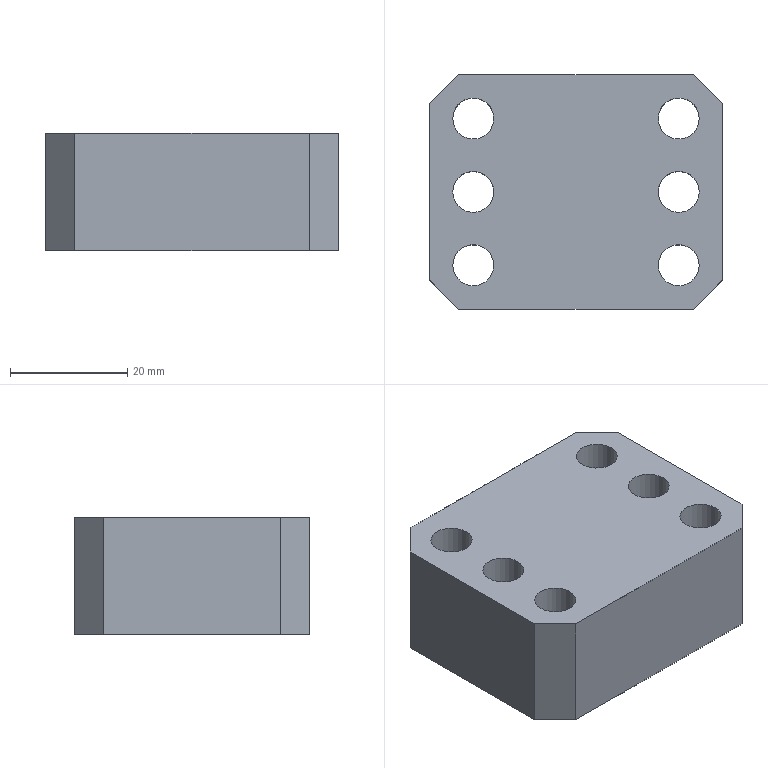Part | NX | features BREP 1 | 1 solid | 16 faces | box 50 x 40 x 20 mm | volume 34382 mm3 | plane 10 | cylinder 6 | commonest cylinder face diameters 7 x6
STEP:
#1=CARTESIAN_POINT('',(25.,-15.,0.));
#2=VERTEX_POINT('',#1);
#3=CARTESIAN_POINT('',(25.,15.,0.));
#4=VERTEX_POINT('',#3);
#5=CARTESIAN_POINT('',(25.,20.,0.));
#6=DIRECTION('',(0.,1.,0.));
#7=VECTOR('',#6,1000.);
#8=LINE('',#5,#7);
#9=EDGE_CURVE('',#2,#4,#8,.T.);
#10=ORIENTED_EDGE('',*,*,#9,.T.);
#11=CARTESIAN_POINT('',(25.,15.,20.));
#12=VERTEX_POINT('',#11);
#13=CARTESIAN_POINT('',(25.,15.,20.));
#14=DIRECTION('',(0.,0.,1.));
#15=VECTOR('',#14,1000.);
#16=LINE('',#13,#15);
#17=EDGE_CURVE('',#4,#12,#16,.T.);
#18=ORIENTED_EDGE('',*,*,#17,.T.);
#19=CARTESIAN_POINT('',(25.,-15.,20.));
#20=VERTEX_POINT('',#19);
#21=CARTESIAN_POINT('',(25.,20.,20.));
#22=DIRECTION('',(0.,1.,0.));
#23=VECTOR('',#22,1000.);
#24=LINE('',#21,#23);
#25=EDGE_CURVE('',#20,#12,#24,.T.);
#26=ORIENTED_EDGE('',*,*,#25,.F.);
#27=CARTESIAN_POINT('',(25.,-15.,20.));
#28=DIRECTION('',(0.,0.,-1.));
#29=VECTOR('',#28,1000.);
#30=LINE('',#27,#29);
#31=EDGE_CURVE('',#20,#2,#30,.T.);
#32=ORIENTED_EDGE('',*,*,#31,.T.);
#33=EDGE_LOOP('',(#10,#18,#26,#32));
#34=FACE_BOUND('',#33,.T.);
#35=CARTESIAN_POINT('',(25.,20.,20.));
#36=DIRECTION('',(-1.,0.,0.));
#37=DIRECTION('',(0.,1.,0.));
#38=AXIS2_PLACEMENT_3D('',#35,#36,#37);
#39=PLANE('',#38);
#40=ADVANCED_FACE('',(#34),#39,.F.);
#41=CARTESIAN_POINT('',(20.,20.,0.));
#42=VERTEX_POINT('',#41);
#43=CARTESIAN_POINT('',(-20.,20.,0.));
#44=VERTEX_POINT('',#43);
#45=CARTESIAN_POINT('',(-25.,20.,0.));
#46=DIRECTION('',(-1.,0.,0.));
#47=VECTOR('',#46,1000.);
#48=LINE('',#45,#47);
#49=EDGE_CURVE('',#42,#44,#48,.T.);
#50=ORIENTED_EDGE('',*,*,#49,.T.);
#51=CARTESIAN_POINT('',(-20.,20.,20.));
#52=VERTEX_POINT('',#51);
#53=CARTESIAN_POINT('',(-20.,20.,20.));
#54=DIRECTION('',(0.,0.,1.));
#55=VECTOR('',#54,1000.);
#56=LINE('',#53,#55);
#57=EDGE_CURVE('',#44,#52,#56,.T.);
#58=ORIENTED_EDGE('',*,*,#57,.T.);
#59=CARTESIAN_POINT('',(20.,20.,20.));
#60=VERTEX_POINT('',#59);
#61=CARTESIAN_POINT('',(-25.,20.,20.));
#62=DIRECTION('',(-1.,0.,0.));
#63=VECTOR('',#62,1000.);
#64=LINE('',#61,#63);
#65=EDGE_CURVE('',#60,#52,#64,.T.);
#66=ORIENTED_EDGE('',*,*,#65,.F.);
#67=CARTESIAN_POINT('',(20.,20.,20.));
#68=DIRECTION('',(0.,0.,-1.));
#69=VECTOR('',#68,1000.);
#70=LINE('',#67,#69);
#71=EDGE_CURVE('',#60,#42,#70,.T.);
#72=ORIENTED_EDGE('',*,*,#71,.T.);
#73=EDGE_LOOP('',(#50,#58,#66,#72));
#74=FACE_BOUND('',#73,.T.);
#75=CARTESIAN_POINT('',(-25.,20.,20.));
#76=DIRECTION('',(0.,-1.,0.));
#77=DIRECTION('',(0.,0.,1.));
#78=AXIS2_PLACEMENT_3D('',#75,#76,#77);
#79=PLANE('',#78);
#80=ADVANCED_FACE('',(#74),#79,.F.);
#81=CARTESIAN_POINT('',(-25.,15.,20.));
#82=VERTEX_POINT('',#81);
#83=CARTESIAN_POINT('',(-25.,-15.,20.));
#84=VERTEX_POINT('',#83);
#85=CARTESIAN_POINT('',(-25.,20.,20.));
#86=DIRECTION('',(0.,-1.,0.));
#87=VECTOR('',#86,1000.);
#88=LINE('',#85,#87);
#89=EDGE_CURVE('',#82,#84,#88,.T.);
#90=ORIENTED_EDGE('',*,*,#89,.F.);
#91=CARTESIAN_POINT('',(-25.,15.,0.));
#92=VERTEX_POINT('',#91);
#93=CARTESIAN_POINT('',(-25.,15.,20.));
#94=DIRECTION('',(0.,0.,-1.));
#95=VECTOR('',#94,1000.);
#96=LINE('',#93,#95);
#97=EDGE_CURVE('',#82,#92,#96,.T.);
#98=ORIENTED_EDGE('',*,*,#97,.T.);
#99=CARTESIAN_POINT('',(-25.,-15.,0.));
#100=VERTEX_POINT('',#99);
#101=CARTESIAN_POINT('',(-25.,20.,0.));
#102=DIRECTION('',(0.,-1.,0.));
#103=VECTOR('',#102,1000.);
#104=LINE('',#101,#103);
#105=EDGE_CURVE('',#92,#100,#104,.T.);
#106=ORIENTED_EDGE('',*,*,#105,.T.);
#107=CARTESIAN_POINT('',(-25.,-15.,20.));
#108=DIRECTION('',(0.,0.,1.));
#109=VECTOR('',#108,1000.);
#110=LINE('',#107,#109);
#111=EDGE_CURVE('',#100,#84,#110,.T.);
#112=ORIENTED_EDGE('',*,*,#111,.T.);
#113=EDGE_LOOP('',(#90,#98,#106,#112));
#114=FACE_BOUND('',#113,.T.);
#115=CARTESIAN_POINT('',(-25.,20.,20.));
#116=DIRECTION('',(1.,0.,0.));
#117=DIRECTION('',(0.,-1.,0.));
#118=AXIS2_PLACEMENT_3D('',#115,#116,#117);
#119=PLANE('',#118);
#120=ADVANCED_FACE('',(#114),#119,.F.);
#121=CARTESIAN_POINT('',(-20.,-20.,20.));
#122=VERTEX_POINT('',#121);
#123=CARTESIAN_POINT('',(20.,-20.,20.));
#124=VERTEX_POINT('',#123);
#125=CARTESIAN_POINT('',(-25.,-20.,20.));
#126=DIRECTION('',(1.,0.,0.));
#127=VECTOR('',#126,1000.);
#128=LINE('',#125,#127);
#129=EDGE_CURVE('',#122,#124,#128,.T.);
#130=ORIENTED_EDGE('',*,*,#129,.F.);
#131=CARTESIAN_POINT('',(-20.,-20.,0.));
#132=VERTEX_POINT('',#131);
#133=CARTESIAN_POINT('',(-20.,-20.,20.));
#134=DIRECTION('',(0.,0.,-1.));
#135=VECTOR('',#134,1000.);
#136=LINE('',#133,#135);
#137=EDGE_CURVE('',#122,#132,#136,.T.);
#138=ORIENTED_EDGE('',*,*,#137,.T.);
#139=CARTESIAN_POINT('',(20.,-20.,0.));
#140=VERTEX_POINT('',#139);
#141=CARTESIAN_POINT('',(-25.,-20.,0.));
#142=DIRECTION('',(1.,0.,0.));
#143=VECTOR('',#142,1000.);
#144=LINE('',#141,#143);
#145=EDGE_CURVE('',#132,#140,#144,.T.);
#146=ORIENTED_EDGE('',*,*,#145,.T.);
#147=CARTESIAN_POINT('',(20.,-20.,20.));
#148=DIRECTION('',(0.,0.,1.));
#149=VECTOR('',#148,1000.);
#150=LINE('',#147,#149);
#151=EDGE_CURVE('',#140,#124,#150,.T.);
#152=ORIENTED_EDGE('',*,*,#151,.T.);
#153=EDGE_LOOP('',(#130,#138,#146,#152));
#154=FACE_BOUND('',#153,.T.);
#155=CARTESIAN_POINT('',(-25.,-20.,20.));
#156=DIRECTION('',(0.,1.,0.));
#157=DIRECTION('',(0.,0.,-1.));
#158=AXIS2_PLACEMENT_3D('',#155,#156,#157);
#159=PLANE('',#158);
#160=ADVANCED_FACE('',(#154),#159,.F.);
#161=CARTESIAN_POINT('',(21.,-12.5,20.));
#162=VERTEX_POINT('',#161);
#163=CARTESIAN_POINT('',(17.5,-12.5,20.));
#164=DIRECTION('',(0.,0.,1.));
#165=DIRECTION('',(1.,0.,0.));
#166=AXIS2_PLACEMENT_3D('',#163,#164,#165);
#167=CIRCLE('',#166,3.5);
#168=EDGE_CURVE('',#162,#162,#167,.T.);
#169=ORIENTED_EDGE('',*,*,#168,.F.);
#170=EDGE_LOOP('',(#169));
#171=FACE_BOUND('',#170,.T.);
#172=CARTESIAN_POINT('',(21.,0.,20.));
#173=VERTEX_POINT('',#172);
#174=CARTESIAN_POINT('',(17.5,0.,20.));
#175=DIRECTION('',(0.,0.,1.));
#176=DIRECTION('',(1.,0.,0.));
#177=AXIS2_PLACEMENT_3D('',#174,#175,#176);
#178=CIRCLE('',#177,3.5);
#179=EDGE_CURVE('',#173,#173,#178,.T.);
#180=ORIENTED_EDGE('',*,*,#179,.F.);
#181=EDGE_LOOP('',(#180));
#182=FACE_BOUND('',#181,.T.);
#183=CARTESIAN_POINT('',(21.,12.5,20.));
#184=VERTEX_POINT('',#183);
#185=CARTESIAN_POINT('',(17.5,12.5,20.));
#186=DIRECTION('',(0.,0.,1.));
#187=DIRECTION('',(1.,0.,0.));
#188=AXIS2_PLACEMENT_3D('',#185,#186,#187);
#189=CIRCLE('',#188,3.5);
#190=EDGE_CURVE('',#184,#184,#189,.T.);
#191=ORIENTED_EDGE('',*,*,#190,.F.);
#192=EDGE_LOOP('',(#191));
#193=FACE_BOUND('',#192,.T.);
#194=CARTESIAN_POINT('',(-14.,12.5,20.));
#195=VERTEX_POINT('',#194);
#196=CARTESIAN_POINT('',(-17.5,12.5,20.));
#197=DIRECTION('',(0.,0.,1.));
#198=DIRECTION('',(1.,0.,0.));
#199=AXIS2_PLACEMENT_3D('',#196,#197,#198);
#200=CIRCLE('',#199,3.5);
#201=EDGE_CURVE('',#195,#195,#200,.T.);
#202=ORIENTED_EDGE('',*,*,#201,.F.);
#203=EDGE_LOOP('',(#202));
#204=FACE_BOUND('',#203,.T.);
#205=CARTESIAN_POINT('',(-14.,0.,20.));
#206=VERTEX_POINT('',#205);
#207=CARTESIAN_POINT('',(-17.5,0.,20.));
#208=DIRECTION('',(0.,0.,1.));
#209=DIRECTION('',(1.,0.,0.));
#210=AXIS2_PLACEMENT_3D('',#207,#208,#209);
#211=CIRCLE('',#210,3.5);
#212=EDGE_CURVE('',#206,#206,#211,.T.);
#213=ORIENTED_EDGE('',*,*,#212,.F.);
#214=EDGE_LOOP('',(#213));
#215=FACE_BOUND('',#214,.T.);
#216=CARTESIAN_POINT('',(-14.,-12.5,20.));
#217=VERTEX_POINT('',#216);
#218=CARTESIAN_POINT('',(-17.5,-12.5,20.));
#219=DIRECTION('',(0.,0.,1.));
#220=DIRECTION('',(1.,0.,0.));
#221=AXIS2_PLACEMENT_3D('',#218,#219,#220);
#222=CIRCLE('',#221,3.5);
#223=EDGE_CURVE('',#217,#217,#222,.T.);
#224=ORIENTED_EDGE('',*,*,#223,.F.);
#225=EDGE_LOOP('',(#224));
#226=FACE_BOUND('',#225,.T.);
#227=ORIENTED_EDGE('',*,*,#65,.T.);
#228=CARTESIAN_POINT('',(-20.,20.,20.));
#229=DIRECTION('',(-0.7071,-0.7071,0.));
#230=VECTOR('',#229,1000.);
#231=LINE('',#228,#230);
#232=EDGE_CURVE('',#52,#82,#231,.T.);
#233=ORIENTED_EDGE('',*,*,#232,.T.);
#234=ORIENTED_EDGE('',*,*,#89,.T.);
#235=CARTESIAN_POINT('',(-20.,-20.,20.));
#236=DIRECTION('',(0.7071,-0.7071,0.));
#237=VECTOR('',#236,1000.);
#238=LINE('',#235,#237);
#239=EDGE_CURVE('',#84,#122,#238,.T.);
#240=ORIENTED_EDGE('',*,*,#239,.T.);
#241=ORIENTED_EDGE('',*,*,#129,.T.);
#242=CARTESIAN_POINT('',(20.,-20.,20.));
#243=DIRECTION('',(0.7071,0.7071,0.));
#244=VECTOR('',#243,1000.);
#245=LINE('',#242,#244);
#246=EDGE_CURVE('',#124,#20,#245,.T.);
#247=ORIENTED_EDGE('',*,*,#246,.T.);
#248=ORIENTED_EDGE('',*,*,#25,.T.);
#249=CARTESIAN_POINT('',(20.,20.,20.));
#250=DIRECTION('',(-0.7071,0.7071,0.));
#251=VECTOR('',#250,1000.);
#252=LINE('',#249,#251);
#253=EDGE_CURVE('',#12,#60,#252,.T.);
#254=ORIENTED_EDGE('',*,*,#253,.T.);
#255=EDGE_LOOP('',(#227,#233,#234,#240,#241,#247,#248,#254));
#256=FACE_BOUND('',#255,.T.);
#257=CARTESIAN_POINT('',(0.,0.,20.));
#258=DIRECTION('',(0.,0.,1.));
#259=DIRECTION('',(-1.,0.,0.));
#260=AXIS2_PLACEMENT_3D('',#257,#258,#259);
#261=PLANE('',#260);
#262=ADVANCED_FACE('',(#171,#182,#193,#204,#215,#226,#256),#261,.T.);
#263=CARTESIAN_POINT('',(21.,-12.5,0.));
#264=VERTEX_POINT('',#263);
#265=CARTESIAN_POINT('',(17.5,-12.5,0.));
#266=DIRECTION('',(0.,0.,1.));
#267=DIRECTION('',(1.,0.,0.));
#268=AXIS2_PLACEMENT_3D('',#265,#266,#267);
#269=CIRCLE('',#268,3.5);
#270=EDGE_CURVE('',#264,#264,#269,.T.);
#271=ORIENTED_EDGE('',*,*,#270,.T.);
#272=EDGE_LOOP('',(#271));
#273=FACE_BOUND('',#272,.T.);
#274=CARTESIAN_POINT('',(21.,0.,0.));
#275=VERTEX_POINT('',#274);
#276=CARTESIAN_POINT('',(17.5,0.,0.));
#277=DIRECTION('',(0.,0.,1.));
#278=DIRECTION('',(1.,0.,0.));
#279=AXIS2_PLACEMENT_3D('',#276,#277,#278);
#280=CIRCLE('',#279,3.5);
#281=EDGE_CURVE('',#275,#275,#280,.T.);
#282=ORIENTED_EDGE('',*,*,#281,.T.);
#283=EDGE_LOOP('',(#282));
#284=FACE_BOUND('',#283,.T.);
#285=CARTESIAN_POINT('',(21.,12.5,0.));
#286=VERTEX_POINT('',#285);
#287=CARTESIAN_POINT('',(17.5,12.5,0.));
#288=DIRECTION('',(0.,0.,1.));
#289=DIRECTION('',(1.,0.,0.));
#290=AXIS2_PLACEMENT_3D('',#287,#288,#289);
#291=CIRCLE('',#290,3.5);
#292=EDGE_CURVE('',#286,#286,#291,.T.);
#293=ORIENTED_EDGE('',*,*,#292,.T.);
#294=EDGE_LOOP('',(#293));
#295=FACE_BOUND('',#294,.T.);
#296=CARTESIAN_POINT('',(-14.,12.5,0.));
#297=VERTEX_POINT('',#296);
#298=CARTESIAN_POINT('',(-17.5,12.5,0.));
#299=DIRECTION('',(0.,0.,1.));
#300=DIRECTION('',(1.,0.,0.));
#301=AXIS2_PLACEMENT_3D('',#298,#299,#300);
#302=CIRCLE('',#301,3.5);
#303=EDGE_CURVE('',#297,#297,#302,.T.);
#304=ORIENTED_EDGE('',*,*,#303,.T.);
#305=EDGE_LOOP('',(#304));
#306=FACE_BOUND('',#305,.T.);
#307=CARTESIAN_POINT('',(-14.,0.,0.));
#308=VERTEX_POINT('',#307);
#309=CARTESIAN_POINT('',(-17.5,0.,0.));
#310=DIRECTION('',(0.,0.,1.));
#311=DIRECTION('',(1.,0.,0.));
#312=AXIS2_PLACEMENT_3D('',#309,#310,#311);
#313=CIRCLE('',#312,3.5);
#314=EDGE_CURVE('',#308,#308,#313,.T.);
#315=ORIENTED_EDGE('',*,*,#314,.T.);
#316=EDGE_LOOP('',(#315));
#317=FACE_BOUND('',#316,.T.);
#318=CARTESIAN_POINT('',(-14.,-12.5,0.));
#319=VERTEX_POINT('',#318);
#320=CARTESIAN_POINT('',(-17.5,-12.5,0.));
#321=DIRECTION('',(0.,0.,1.));
#322=DIRECTION('',(1.,0.,0.));
#323=AXIS2_PLACEMENT_3D('',#320,#321,#322);
#324=CIRCLE('',#323,3.5);
#325=EDGE_CURVE('',#319,#319,#324,.T.);
#326=ORIENTED_EDGE('',*,*,#325,.T.);
#327=EDGE_LOOP('',(#326));
#328=FACE_BOUND('',#327,.T.);
#329=ORIENTED_EDGE('',*,*,#105,.F.);
#330=CARTESIAN_POINT('',(-25.,15.,0.));
#331=DIRECTION('',(0.7071,0.7071,0.));
#332=VECTOR('',#331,1000.);
#333=LINE('',#330,#332);
#334=EDGE_CURVE('',#92,#44,#333,.T.);
#335=ORIENTED_EDGE('',*,*,#334,.T.);
#336=ORIENTED_EDGE('',*,*,#49,.F.);
#337=CARTESIAN_POINT('',(20.,20.,0.));
#338=DIRECTION('',(0.7071,-0.7071,0.));
#339=VECTOR('',#338,1000.);
#340=LINE('',#337,#339);
#341=EDGE_CURVE('',#42,#4,#340,.T.);
#342=ORIENTED_EDGE('',*,*,#341,.T.);
#343=ORIENTED_EDGE('',*,*,#9,.F.);
#344=CARTESIAN_POINT('',(25.,-15.,0.));
#345=DIRECTION('',(-0.7071,-0.7071,0.));
#346=VECTOR('',#345,1000.);
#347=LINE('',#344,#346);
#348=EDGE_CURVE('',#2,#140,#347,.T.);
#349=ORIENTED_EDGE('',*,*,#348,.T.);
#350=ORIENTED_EDGE('',*,*,#145,.F.);
#351=CARTESIAN_POINT('',(-20.,-20.,0.));
#352=DIRECTION('',(-0.7071,0.7071,0.));
#353=VECTOR('',#352,1000.);
#354=LINE('',#351,#353);
#355=EDGE_CURVE('',#132,#100,#354,.T.);
#356=ORIENTED_EDGE('',*,*,#355,.T.);
#357=EDGE_LOOP('',(#329,#335,#336,#342,#343,#349,#350,#356));
#358=FACE_BOUND('',#357,.T.);
#359=CARTESIAN_POINT('',(0.,0.,0.));
#360=DIRECTION('',(0.,0.,1.));
#361=DIRECTION('',(-1.,0.,0.));
#362=AXIS2_PLACEMENT_3D('',#359,#360,#361);
#363=PLANE('',#362);
#364=ADVANCED_FACE('',(#273,#284,#295,#306,#317,#328,#358),#363,.F.);
#365=ORIENTED_EDGE('',*,*,#325,.F.);
#366=EDGE_LOOP('',(#365));
#367=FACE_BOUND('',#366,.T.);
#368=ORIENTED_EDGE('',*,*,#223,.T.);
#369=EDGE_LOOP('',(#368));
#370=FACE_BOUND('',#369,.T.);
#371=CARTESIAN_POINT('',(-17.5,-12.5,20.));
#372=DIRECTION('',(0.,0.,1.));
#373=DIRECTION('',(-1.,0.,0.));
#374=AXIS2_PLACEMENT_3D('',#371,#372,#373);
#375=CYLINDRICAL_SURFACE('',#374,3.5);
#376=ADVANCED_FACE('',(#367,#370),#375,.F.);
#377=ORIENTED_EDGE('',*,*,#314,.F.);
#378=EDGE_LOOP('',(#377));
#379=FACE_BOUND('',#378,.T.);
#380=ORIENTED_EDGE('',*,*,#212,.T.);
#381=EDGE_LOOP('',(#380));
#382=FACE_BOUND('',#381,.T.);
#383=CARTESIAN_POINT('',(-17.5,0.,20.));
#384=DIRECTION('',(0.,0.,1.));
#385=DIRECTION('',(-1.,0.,0.));
#386=AXIS2_PLACEMENT_3D('',#383,#384,#385);
#387=CYLINDRICAL_SURFACE('',#386,3.5);
#388=ADVANCED_FACE('',(#379,#382),#387,.F.);
#389=ORIENTED_EDGE('',*,*,#303,.F.);
#390=EDGE_LOOP('',(#389));
#391=FACE_BOUND('',#390,.T.);
#392=ORIENTED_EDGE('',*,*,#201,.T.);
#393=EDGE_LOOP('',(#392));
#394=FACE_BOUND('',#393,.T.);
#395=CARTESIAN_POINT('',(-17.5,12.5,20.));
#396=DIRECTION('',(0.,0.,1.));
#397=DIRECTION('',(-1.,0.,0.));
#398=AXIS2_PLACEMENT_3D('',#395,#396,#397);
#399=CYLINDRICAL_SURFACE('',#398,3.5);
#400=ADVANCED_FACE('',(#391,#394),#399,.F.);
#401=ORIENTED_EDGE('',*,*,#292,.F.);
#402=EDGE_LOOP('',(#401));
#403=FACE_BOUND('',#402,.T.);
#404=ORIENTED_EDGE('',*,*,#190,.T.);
#405=EDGE_LOOP('',(#404));
#406=FACE_BOUND('',#405,.T.);
#407=CARTESIAN_POINT('',(17.5,12.5,20.));
#408=DIRECTION('',(0.,0.,1.));
#409=DIRECTION('',(-1.,0.,0.));
#410=AXIS2_PLACEMENT_3D('',#407,#408,#409);
#411=CYLINDRICAL_SURFACE('',#410,3.5);
#412=ADVANCED_FACE('',(#403,#406),#411,.F.);
#413=ORIENTED_EDGE('',*,*,#281,.F.);
#414=EDGE_LOOP('',(#413));
#415=FACE_BOUND('',#414,.T.);
#416=ORIENTED_EDGE('',*,*,#179,.T.);
#417=EDGE_LOOP('',(#416));
#418=FACE_BOUND('',#417,.T.);
#419=CARTESIAN_POINT('',(17.5,0.,20.));
#420=DIRECTION('',(0.,0.,1.));
#421=DIRECTION('',(-1.,0.,0.));
#422=AXIS2_PLACEMENT_3D('',#419,#420,#421);
#423=CYLINDRICAL_SURFACE('',#422,3.5);
#424=ADVANCED_FACE('',(#415,#418),#423,.F.);
#425=ORIENTED_EDGE('',*,*,#270,.F.);
#426=EDGE_LOOP('',(#425));
#427=FACE_BOUND('',#426,.T.);
#428=ORIENTED_EDGE('',*,*,#168,.T.);
#429=EDGE_LOOP('',(#428));
#430=FACE_BOUND('',#429,.T.);
#431=CARTESIAN_POINT('',(17.5,-12.5,20.));
#432=DIRECTION('',(0.,0.,1.));
#433=DIRECTION('',(-1.,0.,0.));
#434=AXIS2_PLACEMENT_3D('',#431,#432,#433);
#435=CYLINDRICAL_SURFACE('',#434,3.5);
#436=ADVANCED_FACE('',(#427,#430),#435,.F.);
#437=ORIENTED_EDGE('',*,*,#232,.F.);
#438=ORIENTED_EDGE('',*,*,#57,.F.);
#439=ORIENTED_EDGE('',*,*,#334,.F.);
#440=ORIENTED_EDGE('',*,*,#97,.F.);
#441=EDGE_LOOP('',(#437,#438,#439,#440));
#442=FACE_BOUND('',#441,.T.);
#443=CARTESIAN_POINT('',(-25.,15.,20.));
#444=DIRECTION('',(0.7071,-0.7071,0.));
#445=DIRECTION('',(0.,0.,1.));
#446=AXIS2_PLACEMENT_3D('',#443,#444,#445);
#447=PLANE('',#446);
#448=ADVANCED_FACE('',(#442),#447,.F.);
#449=ORIENTED_EDGE('',*,*,#253,.F.);
#450=ORIENTED_EDGE('',*,*,#17,.F.);
#451=ORIENTED_EDGE('',*,*,#341,.F.);
#452=ORIENTED_EDGE('',*,*,#71,.F.);
#453=EDGE_LOOP('',(#449,#450,#451,#452));
#454=FACE_BOUND('',#453,.T.);
#455=CARTESIAN_POINT('',(20.,20.,20.));
#456=DIRECTION('',(-0.7071,-0.7071,0.));
#457=DIRECTION('',(0.,0.,1.));
#458=AXIS2_PLACEMENT_3D('',#455,#456,#457);
#459=PLANE('',#458);
#460=ADVANCED_FACE('',(#454),#459,.F.);
#461=ORIENTED_EDGE('',*,*,#239,.F.);
#462=ORIENTED_EDGE('',*,*,#111,.F.);
#463=ORIENTED_EDGE('',*,*,#355,.F.);
#464=ORIENTED_EDGE('',*,*,#137,.F.);
#465=EDGE_LOOP('',(#461,#462,#463,#464));
#466=FACE_BOUND('',#465,.T.);
#467=CARTESIAN_POINT('',(-20.,-20.,20.));
#468=DIRECTION('',(0.7071,0.7071,0.));
#469=DIRECTION('',(0.,0.,1.));
#470=AXIS2_PLACEMENT_3D('',#467,#468,#469);
#471=PLANE('',#470);
#472=ADVANCED_FACE('',(#466),#471,.F.);
#473=ORIENTED_EDGE('',*,*,#246,.F.);
#474=ORIENTED_EDGE('',*,*,#151,.F.);
#475=ORIENTED_EDGE('',*,*,#348,.F.);
#476=ORIENTED_EDGE('',*,*,#31,.F.);
#477=EDGE_LOOP('',(#473,#474,#475,#476));
#478=FACE_BOUND('',#477,.T.);
#479=CARTESIAN_POINT('',(25.,-15.,20.));
#480=DIRECTION('',(-0.7071,0.7071,0.));
#481=DIRECTION('',(0.,0.,1.));
#482=AXIS2_PLACEMENT_3D('',#479,#480,#481);
#483=PLANE('',#482);
#484=ADVANCED_FACE('',(#478),#483,.F.);
#485=CLOSED_SHELL('',(#40,#80,#120,#160,#262,#364,#376,#388,#400,#412,#424,#436,#448,#460,#472,#484));
#486=MANIFOLD_SOLID_BREP('',#485);
#487=(LENGTH_UNIT()NAMED_UNIT(*)SI_UNIT(.MILLI.,.METRE.));
#488=UNCERTAINTY_MEASURE_WITH_UNIT(LENGTH_MEASURE(0.00001),#487,'','');
#489=(NAMED_UNIT(*)PLANE_ANGLE_UNIT()SI_UNIT($,.RADIAN.));
#490=(NAMED_UNIT(*)SI_UNIT($,.STERADIAN.)SOLID_ANGLE_UNIT());
#491=(GEOMETRIC_REPRESENTATION_CONTEXT(3)GLOBAL_UNCERTAINTY_ASSIGNED_CONTEXT((#488))GLOBAL_UNIT_ASSIGNED_CONTEXT((#487,#489,#490))REPRESENTATION_CONTEXT('',''));
#492=ADVANCED_BREP_SHAPE_REPRESENTATION('',(#486),#491);